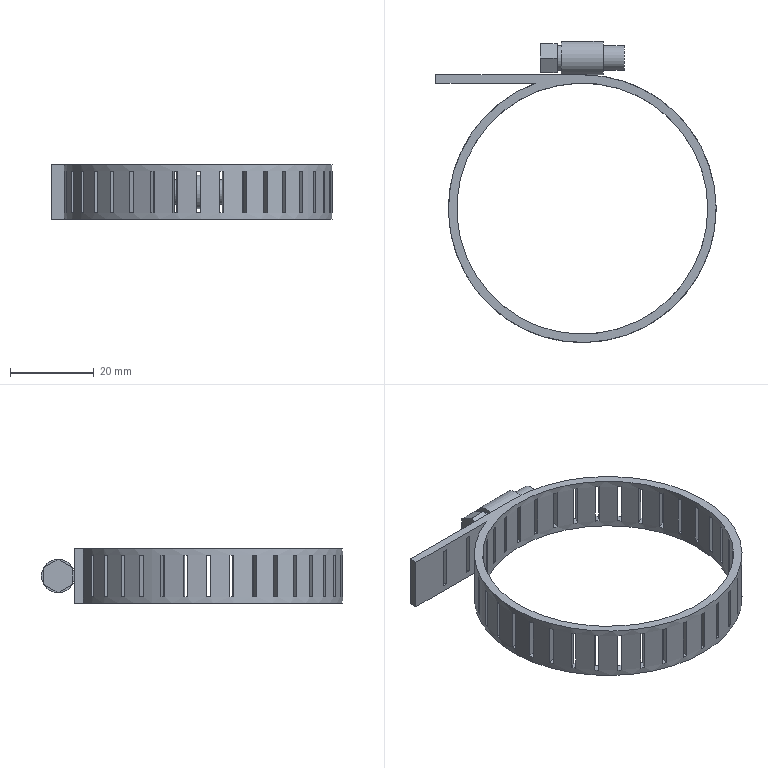Part | STEP file | JBT 8870—1999 70-90 | 3 solids | 181 faces | box 67 x 72 x 13 mm | volume 5818 mm3 | plane 175 | cylinder 6 | commonest cylinder face diameters 5.96 x1 6 x1 8 x1 8.1 x1 60 x1 64 x1